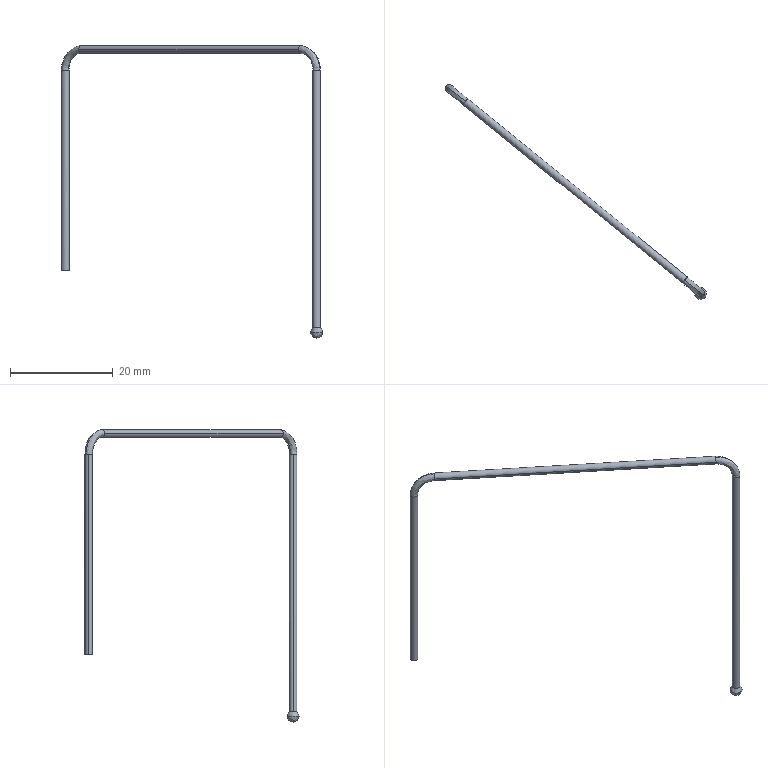Part | SolidWorks | features BaseBody 1 | 1 solid | 13 faces | box 50.783 x 41.654 x 56.908 mm | volume 283.186 mm3 | spline 6 | cylinder 6 | plane 1 | commonest cylinder face diameters 1.5 x6
STEP:
#1=CARTESIAN_POINT('',(557.621,-173.927,280.212));
#2=VERTEX_POINT('',#1);
#3=CARTESIAN_POINT('',(559.121,-173.927,280.212));
#4=VERTEX_POINT('',#3);
#5=CARTESIAN_POINT('',(558.371,-173.927,280.212));
#6=DIRECTION('',(0.000000024,-0.000000004,1.));
#7=DIRECTION('',(-1.,0.,0.000000024));
#8=AXIS2_PLACEMENT_3D('',#5,#6,#7);
#9=CIRCLE('',#8,0.75);
#10=EDGE_CURVE('',#2,#4,#9,.T.);
#11=ORIENTED_EDGE('',*,*,#10,.F.);
#12=CARTESIAN_POINT('',(558.371,-173.927,280.212));
#13=DIRECTION('',(0.000000024,-0.000000004,1.));
#14=DIRECTION('',(-1.,0.,0.000000024));
#15=AXIS2_PLACEMENT_3D('',#12,#13,#14);
#16=CIRCLE('',#15,0.75);
#17=EDGE_CURVE('',#4,#2,#16,.T.);
#18=ORIENTED_EDGE('',*,*,#17,.F.);
#19=EDGE_LOOP('',(#11,#18));
#20=FACE_BOUND('',#19,.T.);
#21=CARTESIAN_POINT('',(557.473,-173.196,279.33));
#22=VERTEX_POINT('',#21);
#23=CARTESIAN_POINT('',(559.269,-174.657,279.33));
#24=VERTEX_POINT('',#23);
#25=CARTESIAN_POINT('',(558.371,-173.927,279.33));
#26=DIRECTION('',(-0.000000024,0.000000004,-1.));
#27=DIRECTION('',(-0.7758,0.6309,0.000000021));
#28=AXIS2_PLACEMENT_3D('',#25,#26,#27);
#29=CIRCLE('',#28,1.158);
#30=EDGE_CURVE('',#22,#24,#29,.T.);
#31=ORIENTED_EDGE('',*,*,#30,.F.);
#32=CARTESIAN_POINT('',(558.371,-173.927,279.33));
#33=DIRECTION('',(0.000000024,-0.000000004,1.));
#34=DIRECTION('',(-0.7758,0.6309,0.000000021));
#35=AXIS2_PLACEMENT_3D('',#32,#33,#34);
#36=CIRCLE('',#35,1.158);
#37=EDGE_CURVE('',#22,#24,#36,.T.);
#38=ORIENTED_EDGE('',*,*,#37,.T.);
#39=EDGE_LOOP('',(#31,#38));
#40=FACE_OUTER_BOUND('',#39,.T.);
#41=CARTESIAN_POINT('',(557.473,-173.196,279.33));
#42=CARTESIAN_POINT('',(557.473,-173.196,279.33));
#43=CARTESIAN_POINT('',(557.473,-173.196,279.33));
#44=CARTESIAN_POINT('',(557.473,-173.196,279.33));
#45=CARTESIAN_POINT('',(556.012,-174.992,279.33));
#46=CARTESIAN_POINT('',(556.012,-174.992,283.96));
#47=CARTESIAN_POINT('',(558.934,-171.4,283.96));
#48=CARTESIAN_POINT('',(558.934,-171.4,279.33));
#49=CARTESIAN_POINT('',(557.808,-176.453,279.33));
#50=CARTESIAN_POINT('',(557.808,-176.453,283.96));
#51=CARTESIAN_POINT('',(560.73,-172.861,283.96));
#52=CARTESIAN_POINT('',(560.73,-172.861,279.33));
#53=CARTESIAN_POINT('',(559.269,-174.657,279.33));
#54=CARTESIAN_POINT('',(559.269,-174.657,279.33));
#55=CARTESIAN_POINT('',(559.269,-174.657,279.33));
#56=CARTESIAN_POINT('',(559.269,-174.657,279.33));
#57=(BOUNDED_SURFACE()B_SPLINE_SURFACE(3,3,((#41,#42,#43,#44),(#45,#46,#47,#48),(#49,#50,#51,#52),(#53,#54,#55,#56)),.UNSPECIFIED.,.F.,.F.,.F.)B_SPLINE_SURFACE_WITH_KNOTS((4,4),(4,4),(0.,1.),(0.,1.),.UNSPECIFIED.)GEOMETRIC_REPRESENTATION_ITEM()RATIONAL_B_SPLINE_SURFACE(((1.,0.3333,0.3333,1.),(0.3333,0.1111,0.1111,0.3333),(0.3333,0.1111,0.1111,0.3333),(1.,0.3333,0.3333,1.)))REPRESENTATION_ITEM('')SURFACE());
#58=ADVANCED_FACE('',(#20,#40),#57,.T.);
#59=CARTESIAN_POINT('',(512.599,-136.704,335.08));
#60=VERTEX_POINT('',#59);
#61=CARTESIAN_POINT('',(512.126,-137.285,334.33));
#62=VERTEX_POINT('',#61);
#63=CARTESIAN_POINT('',(512.599,-136.704,334.33));
#64=DIRECTION('',(0.7758,-0.6309,-0.000000021));
#65=DIRECTION('',(0.6309,0.7758,0.));
#66=AXIS2_PLACEMENT_3D('',#63,#64,#65);
#67=CIRCLE('',#66,0.75);
#68=EDGE_CURVE('',#60,#62,#67,.T.);
#69=ORIENTED_EDGE('',*,*,#68,.T.);
#70=CARTESIAN_POINT('',(554.794,-171.985,334.33));
#71=VERTEX_POINT('',#70);
#72=CARTESIAN_POINT('',(554.794,-171.985,334.33));
#73=DIRECTION('',(0.7758,-0.6309,-0.000000021));
#74=VECTOR('',#73,1000.);
#75=LINE('',#72,#74);
#76=EDGE_CURVE('',#62,#71,#75,.T.);
#77=ORIENTED_EDGE('',*,*,#76,.T.);
#78=CARTESIAN_POINT('',(555.268,-171.403,335.08));
#79=VERTEX_POINT('',#78);
#80=CARTESIAN_POINT('',(555.268,-171.403,334.33));
#81=DIRECTION('',(-0.7758,0.6309,0.000000021));
#82=DIRECTION('',(0.6309,0.7758,0.));
#83=AXIS2_PLACEMENT_3D('',#80,#81,#82);
#84=CIRCLE('',#83,0.75);
#85=EDGE_CURVE('',#71,#79,#84,.T.);
#86=ORIENTED_EDGE('',*,*,#85,.T.);
#87=CARTESIAN_POINT('',(555.741,-170.821,334.33));
#88=VERTEX_POINT('',#87);
#89=CARTESIAN_POINT('',(555.268,-171.403,334.33));
#90=DIRECTION('',(-0.7758,0.6309,0.000000021));
#91=DIRECTION('',(0.6309,0.7758,0.));
#92=AXIS2_PLACEMENT_3D('',#89,#90,#91);
#93=CIRCLE('',#92,0.75);
#94=EDGE_CURVE('',#79,#88,#93,.T.);
#95=ORIENTED_EDGE('',*,*,#94,.T.);
#96=CARTESIAN_POINT('',(513.072,-136.122,334.33));
#97=VERTEX_POINT('',#96);
#98=CARTESIAN_POINT('',(555.741,-170.821,334.33));
#99=DIRECTION('',(0.7758,-0.6309,-0.000000021));
#100=VECTOR('',#99,1000.);
#101=LINE('',#98,#100);
#102=EDGE_CURVE('',#97,#88,#101,.T.);
#103=ORIENTED_EDGE('',*,*,#102,.F.);
#104=CARTESIAN_POINT('',(512.599,-136.704,334.33));
#105=DIRECTION('',(0.7758,-0.6309,-0.000000021));
#106=DIRECTION('',(0.6309,0.7758,0.));
#107=AXIS2_PLACEMENT_3D('',#104,#105,#106);
#108=CIRCLE('',#107,0.75);
#109=EDGE_CURVE('',#97,#60,#108,.T.);
#110=ORIENTED_EDGE('',*,*,#109,.T.);
#111=EDGE_LOOP('',(#69,#77,#86,#95,#103,#110));
#112=FACE_OUTER_BOUND('',#111,.T.);
#113=CARTESIAN_POINT('',(555.268,-171.403,334.33));
#114=DIRECTION('',(0.7758,-0.6309,-0.000000021));
#115=DIRECTION('',(0.6309,0.7758,0.));
#116=AXIS2_PLACEMENT_3D('',#113,#114,#115);
#117=CYLINDRICAL_SURFACE('',#116,0.75);
#118=ADVANCED_FACE('',(#112),#117,.T.);
#119=CARTESIAN_POINT('',(508.745,-134.18,330.33));
#120=VERTEX_POINT('',#119);
#121=CARTESIAN_POINT('',(510.077,-134.653,330.33));
#122=VERTEX_POINT('',#121);
#123=CARTESIAN_POINT('',(509.495,-134.18,330.33));
#124=DIRECTION('',(0.000000024,-0.000000004,1.));
#125=DIRECTION('',(-0.7758,0.6309,0.000000021));
#126=AXIS2_PLACEMENT_3D('',#123,#124,#125);
#127=CIRCLE('',#126,0.75);
#128=EDGE_CURVE('',#120,#122,#127,.T.);
#129=ORIENTED_EDGE('',*,*,#128,.T.);
#130=CARTESIAN_POINT('',(512.599,-136.704,333.58));
#131=VERTEX_POINT('',#130);
#132=CARTESIAN_POINT('',(512.599,-136.704,330.33));
#133=DIRECTION('',(0.6309,0.7758,-0.000000012));
#134=DIRECTION('',(0.000000024,-0.000000004,1.));
#135=AXIS2_PLACEMENT_3D('',#132,#133,#134);
#136=CIRCLE('',#135,3.25);
#137=EDGE_CURVE('',#122,#131,#136,.T.);
#138=ORIENTED_EDGE('',*,*,#137,.T.);
#139=CARTESIAN_POINT('',(512.599,-136.704,334.33));
#140=DIRECTION('',(0.7758,-0.6309,-0.000000021));
#141=DIRECTION('',(0.6309,0.7758,0.));
#142=AXIS2_PLACEMENT_3D('',#139,#140,#141);
#143=CIRCLE('',#142,0.75);
#144=EDGE_CURVE('',#62,#131,#143,.T.);
#145=ORIENTED_EDGE('',*,*,#144,.F.);
#146=ORIENTED_EDGE('',*,*,#68,.F.);
#147=CARTESIAN_POINT('',(508.914,-133.707,330.33));
#148=VERTEX_POINT('',#147);
#149=CARTESIAN_POINT('',(512.599,-136.704,330.33));
#150=DIRECTION('',(0.6309,0.7758,-0.000000012));
#151=DIRECTION('',(0.000000024,-0.000000004,1.));
#152=AXIS2_PLACEMENT_3D('',#149,#150,#151);
#153=CIRCLE('',#152,4.75);
#154=EDGE_CURVE('',#148,#60,#153,.T.);
#155=ORIENTED_EDGE('',*,*,#154,.F.);
#156=CARTESIAN_POINT('',(509.495,-134.18,330.33));
#157=DIRECTION('',(0.000000024,-0.000000004,1.));
#158=DIRECTION('',(-0.7758,0.6309,0.000000021));
#159=AXIS2_PLACEMENT_3D('',#156,#157,#158);
#160=CIRCLE('',#159,0.75);
#161=EDGE_CURVE('',#148,#120,#160,.T.);
#162=ORIENTED_EDGE('',*,*,#161,.T.);
#163=EDGE_LOOP('',(#129,#138,#145,#146,#155,#162));
#164=FACE_OUTER_BOUND('',#163,.T.);
#165=CARTESIAN_POINT('',(508.914,-133.707,330.33));
#166=CARTESIAN_POINT('',(508.914,-133.707,333.113));
#167=CARTESIAN_POINT('',(510.44,-134.948,335.08));
#168=CARTESIAN_POINT('',(512.599,-136.704,335.08));
#169=CARTESIAN_POINT('',(507.967,-134.87,330.33));
#170=CARTESIAN_POINT('',(507.967,-134.87,333.113));
#171=CARTESIAN_POINT('',(509.494,-136.112,335.08));
#172=CARTESIAN_POINT('',(511.652,-137.867,335.08));
#173=CARTESIAN_POINT('',(509.131,-135.817,330.33));
#174=CARTESIAN_POINT('',(509.131,-135.817,332.234));
#175=CARTESIAN_POINT('',(510.175,-136.666,333.58));
#176=CARTESIAN_POINT('',(511.652,-137.867,333.58));
#177=CARTESIAN_POINT('',(510.077,-134.653,330.33));
#178=CARTESIAN_POINT('',(510.077,-134.653,332.234));
#179=CARTESIAN_POINT('',(511.122,-135.502,333.58));
#180=CARTESIAN_POINT('',(512.599,-136.704,333.58));
#181=(BOUNDED_SURFACE()B_SPLINE_SURFACE(3,3,((#165,#166,#167,#168),(#169,#170,#171,#172),(#173,#174,#175,#176),(#177,#178,#179,#180)),.UNSPECIFIED.,.F.,.F.,.F.)B_SPLINE_SURFACE_WITH_KNOTS((4,4),(4,4),(0.,1.),(0.,1.),.UNSPECIFIED.)GEOMETRIC_REPRESENTATION_ITEM()RATIONAL_B_SPLINE_SURFACE(((1.,0.8047,0.8047,1.),(0.3333,0.2682,0.2682,0.3333),(0.3333,0.2682,0.2682,0.3333),(1.,0.8047,0.8047,1.)))REPRESENTATION_ITEM('')SURFACE());
#182=ADVANCED_FACE('',(#164),#181,.T.);
#183=CARTESIAN_POINT('',(555.268,-171.403,333.58));
#184=VERTEX_POINT('',#183);
#185=CARTESIAN_POINT('',(555.268,-171.403,334.33));
#186=DIRECTION('',(-0.7758,0.6309,0.000000021));
#187=DIRECTION('',(0.6309,0.7758,0.));
#188=AXIS2_PLACEMENT_3D('',#185,#186,#187);
#189=CIRCLE('',#188,0.75);
#190=EDGE_CURVE('',#184,#71,#189,.T.);
#191=ORIENTED_EDGE('',*,*,#190,.F.);
#192=CARTESIAN_POINT('',(557.789,-173.453,330.33));
#193=VERTEX_POINT('',#192);
#194=CARTESIAN_POINT('',(555.268,-171.403,330.33));
#195=DIRECTION('',(0.6309,0.7758,-0.000000012));
#196=DIRECTION('',(0.000000024,-0.000000004,1.));
#197=AXIS2_PLACEMENT_3D('',#194,#195,#196);
#198=CIRCLE('',#197,3.25);
#199=EDGE_CURVE('',#184,#193,#198,.T.);
#200=ORIENTED_EDGE('',*,*,#199,.T.);
#201=CARTESIAN_POINT('',(557.621,-173.927,330.33));
#202=VERTEX_POINT('',#201);
#203=CARTESIAN_POINT('',(558.371,-173.927,330.33));
#204=DIRECTION('',(0.000000024,-0.000000004,1.));
#205=DIRECTION('',(0.7758,-0.6309,-0.000000021));
#206=AXIS2_PLACEMENT_3D('',#203,#204,#205);
#207=CIRCLE('',#206,0.75);
#208=EDGE_CURVE('',#193,#202,#207,.T.);
#209=ORIENTED_EDGE('',*,*,#208,.T.);
#210=CARTESIAN_POINT('',(558.953,-174.4,330.33));
#211=VERTEX_POINT('',#210);
#212=CARTESIAN_POINT('',(558.371,-173.927,330.33));
#213=DIRECTION('',(0.000000024,-0.000000004,1.));
#214=DIRECTION('',(0.7758,-0.6309,-0.000000021));
#215=AXIS2_PLACEMENT_3D('',#212,#213,#214);
#216=CIRCLE('',#215,0.75);
#217=EDGE_CURVE('',#202,#211,#216,.T.);
#218=ORIENTED_EDGE('',*,*,#217,.T.);
#219=CARTESIAN_POINT('',(555.268,-171.403,330.33));
#220=DIRECTION('',(0.6309,0.7758,-0.000000012));
#221=DIRECTION('',(0.000000024,-0.000000004,1.));
#222=AXIS2_PLACEMENT_3D('',#219,#220,#221);
#223=CIRCLE('',#222,4.75);
#224=EDGE_CURVE('',#79,#211,#223,.T.);
#225=ORIENTED_EDGE('',*,*,#224,.F.);
#226=ORIENTED_EDGE('',*,*,#85,.F.);
#227=EDGE_LOOP('',(#191,#200,#209,#218,#225,#226));
#228=FACE_OUTER_BOUND('',#227,.T.);
#229=CARTESIAN_POINT('',(555.268,-171.403,335.08));
#230=CARTESIAN_POINT('',(557.426,-173.158,335.08));
#231=CARTESIAN_POINT('',(558.953,-174.4,333.113));
#232=CARTESIAN_POINT('',(558.953,-174.4,330.33));
#233=CARTESIAN_POINT('',(554.321,-172.567,335.08));
#234=CARTESIAN_POINT('',(556.48,-174.322,335.08));
#235=CARTESIAN_POINT('',(558.006,-175.564,333.113));
#236=CARTESIAN_POINT('',(558.006,-175.564,330.33));
#237=CARTESIAN_POINT('',(554.321,-172.567,333.58));
#238=CARTESIAN_POINT('',(555.798,-173.768,333.58));
#239=CARTESIAN_POINT('',(556.843,-174.617,332.234));
#240=CARTESIAN_POINT('',(556.843,-174.617,330.33));
#241=CARTESIAN_POINT('',(555.268,-171.403,333.58));
#242=CARTESIAN_POINT('',(556.745,-172.604,333.58));
#243=CARTESIAN_POINT('',(557.789,-173.453,332.234));
#244=CARTESIAN_POINT('',(557.789,-173.453,330.33));
#245=(BOUNDED_SURFACE()B_SPLINE_SURFACE(3,3,((#229,#230,#231,#232),(#233,#234,#235,#236),(#237,#238,#239,#240),(#241,#242,#243,#244)),.UNSPECIFIED.,.F.,.F.,.F.)B_SPLINE_SURFACE_WITH_KNOTS((4,4),(4,4),(0.,1.),(0.,1.),.UNSPECIFIED.)GEOMETRIC_REPRESENTATION_ITEM()RATIONAL_B_SPLINE_SURFACE(((1.,0.8047,0.8047,1.),(0.3333,0.2682,0.2682,0.3333),(0.3333,0.2682,0.2682,0.3333),(1.,0.8047,0.8047,1.)))REPRESENTATION_ITEM('')SURFACE());
#246=ADVANCED_FACE('',(#228),#245,.T.);
#247=CARTESIAN_POINT('',(510.245,-134.18,291.293));
#248=VERTEX_POINT('',#247);
#249=CARTESIAN_POINT('',(508.745,-134.18,291.293));
#250=VERTEX_POINT('',#249);
#251=CARTESIAN_POINT('',(509.495,-134.18,291.293));
#252=DIRECTION('',(0.000000024,-0.000000004,1.));
#253=DIRECTION('',(1.,0.,-0.000000024));
#254=AXIS2_PLACEMENT_3D('',#251,#252,#253);
#255=CIRCLE('',#254,0.75);
#256=EDGE_CURVE('',#248,#250,#255,.T.);
#257=ORIENTED_EDGE('',*,*,#256,.T.);
#258=CARTESIAN_POINT('',(508.745,-134.18,330.33));
#259=DIRECTION('',(0.000000024,-0.000000004,1.));
#260=VECTOR('',#259,1000.);
#261=LINE('',#258,#260);
#262=EDGE_CURVE('',#250,#120,#261,.T.);
#263=ORIENTED_EDGE('',*,*,#262,.T.);
#264=ORIENTED_EDGE('',*,*,#161,.F.);
#265=CARTESIAN_POINT('',(510.245,-134.18,330.33));
#266=VERTEX_POINT('',#265);
#267=CARTESIAN_POINT('',(509.495,-134.18,330.33));
#268=DIRECTION('',(0.000000024,-0.000000004,1.));
#269=DIRECTION('',(-0.7758,0.6309,0.000000021));
#270=AXIS2_PLACEMENT_3D('',#267,#268,#269);
#271=CIRCLE('',#270,0.75);
#272=EDGE_CURVE('',#266,#148,#271,.T.);
#273=ORIENTED_EDGE('',*,*,#272,.F.);
#274=CARTESIAN_POINT('',(510.245,-134.18,330.33));
#275=DIRECTION('',(0.000000024,-0.000000004,1.));
#276=VECTOR('',#275,1000.);
#277=LINE('',#274,#276);
#278=EDGE_CURVE('',#248,#266,#277,.T.);
#279=ORIENTED_EDGE('',*,*,#278,.F.);
#280=EDGE_LOOP('',(#257,#263,#264,#273,#279));
#281=FACE_OUTER_BOUND('',#280,.T.);
#282=CARTESIAN_POINT('',(509.495,-134.18,330.33));
#283=DIRECTION('',(0.000000024,-0.000000004,1.));
#284=DIRECTION('',(1.,0.,-0.000000024));
#285=AXIS2_PLACEMENT_3D('',#282,#283,#284);
#286=CYLINDRICAL_SURFACE('',#285,0.75);
#287=ADVANCED_FACE('',(#281),#286,.T.);
#288=CARTESIAN_POINT('',(559.121,-173.927,330.33));
#289=VERTEX_POINT('',#288);
#290=CARTESIAN_POINT('',(558.371,-173.927,330.33));
#291=DIRECTION('',(0.000000024,-0.000000004,1.));
#292=DIRECTION('',(0.7758,-0.6309,-0.000000021));
#293=AXIS2_PLACEMENT_3D('',#290,#291,#292);
#294=CIRCLE('',#293,0.75);
#295=EDGE_CURVE('',#289,#193,#294,.T.);
#296=ORIENTED_EDGE('',*,*,#295,.F.);
#297=CARTESIAN_POINT('',(559.121,-173.927,279.33));
#298=DIRECTION('',(-0.000000024,0.000000004,-1.));
#299=VECTOR('',#298,1000.);
#300=LINE('',#297,#299);
#301=EDGE_CURVE('',#289,#4,#300,.T.);
#302=ORIENTED_EDGE('',*,*,#301,.T.);
#303=ORIENTED_EDGE('',*,*,#17,.T.);
#304=CARTESIAN_POINT('',(557.621,-173.927,279.33));
#305=DIRECTION('',(-0.000000024,0.000000004,-1.));
#306=VECTOR('',#305,1000.);
#307=LINE('',#304,#306);
#308=EDGE_CURVE('',#202,#2,#307,.T.);
#309=ORIENTED_EDGE('',*,*,#308,.F.);
#310=ORIENTED_EDGE('',*,*,#208,.F.);
#311=EDGE_LOOP('',(#296,#302,#303,#309,#310));
#312=FACE_OUTER_BOUND('',#311,.T.);
#313=CARTESIAN_POINT('',(558.371,-173.927,279.33));
#314=DIRECTION('',(-0.000000024,0.000000004,-1.));
#315=DIRECTION('',(-1.,0.,0.000000024));
#316=AXIS2_PLACEMENT_3D('',#313,#314,#315);
#317=CYLINDRICAL_SURFACE('',#316,0.75);
#318=ADVANCED_FACE('',(#312),#317,.T.);
#319=ORIENTED_EDGE('',*,*,#76,.F.);
#320=ORIENTED_EDGE('',*,*,#144,.T.);
#321=CARTESIAN_POINT('',(512.599,-136.704,334.33));
#322=DIRECTION('',(0.7758,-0.6309,-0.000000021));
#323=DIRECTION('',(0.6309,0.7758,0.));
#324=AXIS2_PLACEMENT_3D('',#321,#322,#323);
#325=CIRCLE('',#324,0.75);
#326=EDGE_CURVE('',#131,#97,#325,.T.);
#327=ORIENTED_EDGE('',*,*,#326,.T.);
#328=ORIENTED_EDGE('',*,*,#102,.T.);
#329=CARTESIAN_POINT('',(555.268,-171.403,334.33));
#330=DIRECTION('',(-0.7758,0.6309,0.000000021));
#331=DIRECTION('',(0.6309,0.7758,0.));
#332=AXIS2_PLACEMENT_3D('',#329,#330,#331);
#333=CIRCLE('',#332,0.75);
#334=EDGE_CURVE('',#88,#184,#333,.T.);
#335=ORIENTED_EDGE('',*,*,#334,.T.);
#336=ORIENTED_EDGE('',*,*,#190,.T.);
#337=EDGE_LOOP('',(#319,#320,#327,#328,#335,#336));
#338=FACE_OUTER_BOUND('',#337,.T.);
#339=CARTESIAN_POINT('',(555.268,-171.403,334.33));
#340=DIRECTION('',(0.7758,-0.6309,-0.000000021));
#341=DIRECTION('',(0.6309,0.7758,0.));
#342=AXIS2_PLACEMENT_3D('',#339,#340,#341);
#343=CYLINDRICAL_SURFACE('',#342,0.75);
#344=ADVANCED_FACE('',(#338),#343,.T.);
#345=ORIENTED_EDGE('',*,*,#137,.F.);
#346=CARTESIAN_POINT('',(509.495,-134.18,330.33));
#347=DIRECTION('',(0.000000024,-0.000000004,1.));
#348=DIRECTION('',(-0.7758,0.6309,0.000000021));
#349=AXIS2_PLACEMENT_3D('',#346,#347,#348);
#350=CIRCLE('',#349,0.75);
#351=EDGE_CURVE('',#122,#266,#350,.T.);
#352=ORIENTED_EDGE('',*,*,#351,.T.);
#353=ORIENTED_EDGE('',*,*,#272,.T.);
#354=ORIENTED_EDGE('',*,*,#154,.T.);
#355=ORIENTED_EDGE('',*,*,#109,.F.);
#356=ORIENTED_EDGE('',*,*,#326,.F.);
#357=EDGE_LOOP('',(#345,#352,#353,#354,#355,#356));
#358=FACE_OUTER_BOUND('',#357,.T.);
#359=CARTESIAN_POINT('',(510.077,-134.653,330.33));
#360=CARTESIAN_POINT('',(510.077,-134.653,332.234));
#361=CARTESIAN_POINT('',(511.122,-135.502,333.58));
#362=CARTESIAN_POINT('',(512.599,-136.704,333.58));
#363=CARTESIAN_POINT('',(511.024,-133.489,330.33));
#364=CARTESIAN_POINT('',(511.024,-133.489,332.234));
#365=CARTESIAN_POINT('',(512.068,-134.339,333.58));
#366=CARTESIAN_POINT('',(513.545,-135.54,333.58));
#367=CARTESIAN_POINT('',(509.86,-132.543,330.33));
#368=CARTESIAN_POINT('',(509.86,-132.543,333.113));
#369=CARTESIAN_POINT('',(511.386,-133.784,335.08));
#370=CARTESIAN_POINT('',(513.545,-135.54,335.08));
#371=CARTESIAN_POINT('',(508.914,-133.707,330.33));
#372=CARTESIAN_POINT('',(508.914,-133.707,333.113));
#373=CARTESIAN_POINT('',(510.44,-134.948,335.08));
#374=CARTESIAN_POINT('',(512.599,-136.704,335.08));
#375=(BOUNDED_SURFACE()B_SPLINE_SURFACE(3,3,((#359,#360,#361,#362),(#363,#364,#365,#366),(#367,#368,#369,#370),(#371,#372,#373,#374)),.UNSPECIFIED.,.F.,.F.,.F.)B_SPLINE_SURFACE_WITH_KNOTS((4,4),(4,4),(0.,1.),(0.,1.),.UNSPECIFIED.)GEOMETRIC_REPRESENTATION_ITEM()RATIONAL_B_SPLINE_SURFACE(((1.,0.8047,0.8047,1.),(0.3333,0.2682,0.2682,0.3333),(0.3333,0.2682,0.2682,0.3333),(1.,0.8047,0.8047,1.)))REPRESENTATION_ITEM('')SURFACE());
#376=ADVANCED_FACE('',(#358),#375,.T.);
#377=ORIENTED_EDGE('',*,*,#199,.F.);
#378=ORIENTED_EDGE('',*,*,#334,.F.);
#379=ORIENTED_EDGE('',*,*,#94,.F.);
#380=ORIENTED_EDGE('',*,*,#224,.T.);
#381=CARTESIAN_POINT('',(558.371,-173.927,330.33));
#382=DIRECTION('',(0.000000024,-0.000000004,1.));
#383=DIRECTION('',(0.7758,-0.6309,-0.000000021));
#384=AXIS2_PLACEMENT_3D('',#381,#382,#383);
#385=CIRCLE('',#384,0.75);
#386=EDGE_CURVE('',#211,#289,#385,.T.);
#387=ORIENTED_EDGE('',*,*,#386,.T.);
#388=ORIENTED_EDGE('',*,*,#295,.T.);
#389=EDGE_LOOP('',(#377,#378,#379,#380,#387,#388));
#390=FACE_OUTER_BOUND('',#389,.T.);
#391=CARTESIAN_POINT('',(555.268,-171.403,333.58));
#392=CARTESIAN_POINT('',(556.745,-172.604,333.58));
#393=CARTESIAN_POINT('',(557.789,-173.453,332.234));
#394=CARTESIAN_POINT('',(557.789,-173.453,330.33));
#395=CARTESIAN_POINT('',(556.214,-170.239,333.58));
#396=CARTESIAN_POINT('',(557.691,-171.44,333.58));
#397=CARTESIAN_POINT('',(558.736,-172.29,332.234));
#398=CARTESIAN_POINT('',(558.736,-172.29,330.33));
#399=CARTESIAN_POINT('',(556.214,-170.239,335.08));
#400=CARTESIAN_POINT('',(558.373,-171.995,335.08));
#401=CARTESIAN_POINT('',(559.899,-173.236,333.113));
#402=CARTESIAN_POINT('',(559.899,-173.236,330.33));
#403=CARTESIAN_POINT('',(555.268,-171.403,335.08));
#404=CARTESIAN_POINT('',(557.426,-173.158,335.08));
#405=CARTESIAN_POINT('',(558.953,-174.4,333.113));
#406=CARTESIAN_POINT('',(558.953,-174.4,330.33));
#407=(BOUNDED_SURFACE()B_SPLINE_SURFACE(3,3,((#391,#392,#393,#394),(#395,#396,#397,#398),(#399,#400,#401,#402),(#403,#404,#405,#406)),.UNSPECIFIED.,.F.,.F.,.F.)B_SPLINE_SURFACE_WITH_KNOTS((4,4),(4,4),(0.,1.),(0.,1.),.UNSPECIFIED.)GEOMETRIC_REPRESENTATION_ITEM()RATIONAL_B_SPLINE_SURFACE(((1.,0.8047,0.8047,1.),(0.3333,0.2682,0.2682,0.3333),(0.3333,0.2682,0.2682,0.3333),(1.,0.8047,0.8047,1.)))REPRESENTATION_ITEM('')SURFACE());
#408=ADVANCED_FACE('',(#390),#407,.T.);
#409=ORIENTED_EDGE('',*,*,#262,.F.);
#410=CARTESIAN_POINT('',(509.495,-134.18,291.293));
#411=DIRECTION('',(0.000000024,-0.000000004,1.));
#412=DIRECTION('',(1.,0.,-0.000000024));
#413=AXIS2_PLACEMENT_3D('',#410,#411,#412);
#414=CIRCLE('',#413,0.75);
#415=EDGE_CURVE('',#250,#248,#414,.T.);
#416=ORIENTED_EDGE('',*,*,#415,.T.);
#417=ORIENTED_EDGE('',*,*,#278,.T.);
#418=ORIENTED_EDGE('',*,*,#351,.F.);
#419=ORIENTED_EDGE('',*,*,#128,.F.);
#420=EDGE_LOOP('',(#409,#416,#417,#418,#419));
#421=FACE_OUTER_BOUND('',#420,.T.);
#422=CARTESIAN_POINT('',(509.495,-134.18,330.33));
#423=DIRECTION('',(0.000000024,-0.000000004,1.));
#424=DIRECTION('',(1.,0.,-0.000000024));
#425=AXIS2_PLACEMENT_3D('',#422,#423,#424);
#426=CYLINDRICAL_SURFACE('',#425,0.75);
#427=ADVANCED_FACE('',(#421),#426,.T.);
#428=ORIENTED_EDGE('',*,*,#301,.F.);
#429=ORIENTED_EDGE('',*,*,#386,.F.);
#430=ORIENTED_EDGE('',*,*,#217,.F.);
#431=ORIENTED_EDGE('',*,*,#308,.T.);
#432=ORIENTED_EDGE('',*,*,#10,.T.);
#433=EDGE_LOOP('',(#428,#429,#430,#431,#432));
#434=FACE_OUTER_BOUND('',#433,.T.);
#435=CARTESIAN_POINT('',(558.371,-173.927,279.33));
#436=DIRECTION('',(-0.000000024,0.000000004,-1.));
#437=DIRECTION('',(-1.,0.,0.000000024));
#438=AXIS2_PLACEMENT_3D('',#435,#436,#437);
#439=CYLINDRICAL_SURFACE('',#438,0.75);
#440=ADVANCED_FACE('',(#434),#439,.T.);
#441=ORIENTED_EDGE('',*,*,#256,.F.);
#442=ORIENTED_EDGE('',*,*,#415,.F.);
#443=EDGE_LOOP('',(#441,#442));
#444=FACE_OUTER_BOUND('',#443,.T.);
#445=CARTESIAN_POINT('',(509.495,-134.18,291.293));
#446=DIRECTION('',(-0.000000024,0.000000004,-1.));
#447=DIRECTION('',(-1.,0.,0.000000024));
#448=AXIS2_PLACEMENT_3D('',#445,#446,#447);
#449=PLANE('',#448);
#450=ADVANCED_FACE('',(#444),#449,.T.);
#451=ORIENTED_EDGE('',*,*,#37,.F.);
#452=ORIENTED_EDGE('',*,*,#30,.T.);
#453=EDGE_LOOP('',(#451,#452));
#454=FACE_OUTER_BOUND('',#453,.T.);
#455=CARTESIAN_POINT('',(557.473,-173.196,279.33));
#456=CARTESIAN_POINT('',(557.473,-173.196,279.33));
#457=CARTESIAN_POINT('',(557.473,-173.196,279.33));
#458=CARTESIAN_POINT('',(557.473,-173.196,279.33));
#459=CARTESIAN_POINT('',(558.934,-171.4,279.33));
#460=CARTESIAN_POINT('',(558.934,-171.4,274.7));
#461=CARTESIAN_POINT('',(556.012,-174.992,274.7));
#462=CARTESIAN_POINT('',(556.012,-174.992,279.33));
#463=CARTESIAN_POINT('',(560.73,-172.861,279.33));
#464=CARTESIAN_POINT('',(560.73,-172.861,274.7));
#465=CARTESIAN_POINT('',(557.808,-176.453,274.7));
#466=CARTESIAN_POINT('',(557.808,-176.453,279.33));
#467=CARTESIAN_POINT('',(559.269,-174.657,279.33));
#468=CARTESIAN_POINT('',(559.269,-174.657,279.33));
#469=CARTESIAN_POINT('',(559.269,-174.657,279.33));
#470=CARTESIAN_POINT('',(559.269,-174.657,279.33));
#471=(BOUNDED_SURFACE()B_SPLINE_SURFACE(3,3,((#455,#456,#457,#458),(#459,#460,#461,#462),(#463,#464,#465,#466),(#467,#468,#469,#470)),.UNSPECIFIED.,.F.,.F.,.F.)B_SPLINE_SURFACE_WITH_KNOTS((4,4),(4,4),(0.,1.),(0.,1.),.UNSPECIFIED.)GEOMETRIC_REPRESENTATION_ITEM()RATIONAL_B_SPLINE_SURFACE(((1.,0.3333,0.3333,1.),(0.3333,0.1111,0.1111,0.3333),(0.3333,0.1111,0.1111,0.3333),(1.,0.3333,0.3333,1.)))REPRESENTATION_ITEM('')SURFACE());
#472=ADVANCED_FACE('',(#454),#471,.T.);
#473=CLOSED_SHELL('',(#58,#118,#182,#246,#287,#318,#344,#376,#408,#427,#440,#450,#472));
#474=MANIFOLD_SOLID_BREP('',#473);
#475=CARTESIAN_POINT('',(0.,0.,0.));
#476=DIRECTION('',(0.,0.,1.));
#477=DIRECTION('',(1.,0.,0.));
#478=AXIS2_PLACEMENT_3D('',#475,#476,#477);
#479=(LENGTH_UNIT()NAMED_UNIT(*)SI_UNIT(.MILLI.,.METRE.));
#480=UNCERTAINTY_MEASURE_WITH_UNIT(LENGTH_MEASURE(0.00001),#479,'','');
#481=(NAMED_UNIT(*)PLANE_ANGLE_UNIT()SI_UNIT($,.RADIAN.));
#482=(NAMED_UNIT(*)SI_UNIT($,.STERADIAN.)SOLID_ANGLE_UNIT());
#483=(GEOMETRIC_REPRESENTATION_CONTEXT(3)GLOBAL_UNCERTAINTY_ASSIGNED_CONTEXT((#480))GLOBAL_UNIT_ASSIGNED_CONTEXT((#479,#481,#482))REPRESENTATION_CONTEXT('',''));
#484=ADVANCED_BREP_SHAPE_REPRESENTATION('',(#474,#478),#483);